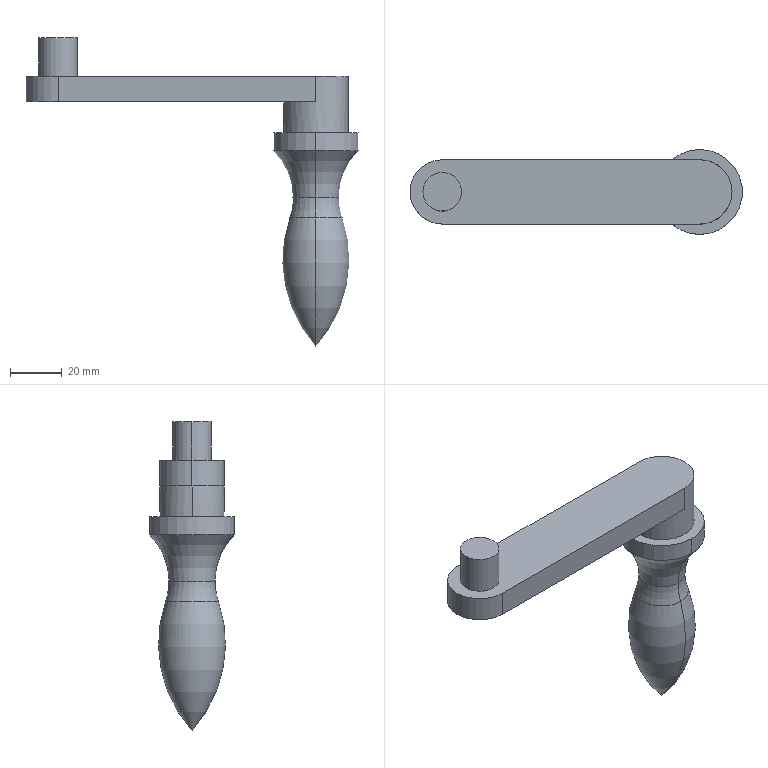Part | SolidWorks | features Extrusion 1, ICE 1, Revolution 1 | 1 solid | 20 faces | box 129 x 33 x 119.886 mm | volume 71552 mm3 | cylinder 8 | torus 6 | plane 6 | commonest cylinder face diameters 25 x4 15 x2 33 x2
STEP:
#1=CARTESIAN_POINT('',(100.,-4.,-19.));
#2=VERTEX_POINT('',#1);
#3=CARTESIAN_POINT('',(100.,3.558,-36.917));
#4=VERTEX_POINT('',#3);
#5=CARTESIAN_POINT('',(100.,-21.456,-36.917));
#6=DIRECTION('',(-1.,0.,0.));
#7=DIRECTION('',(0.,0.,1.));
#8=AXIS2_PLACEMENT_3D('',#5,#6,#7);
#9=CIRCLE('',#8,25.014);
#10=EDGE_CURVE('',#2,#4,#9,.T.);
#11=ORIENTED_EDGE('',*,*,#10,.T.);
#12=CARTESIAN_POINT('',(100.,21.442,-36.917));
#13=VERTEX_POINT('',#12);
#14=CARTESIAN_POINT('',(100.,12.5,-36.917));
#15=DIRECTION('',(0.,0.,1.));
#16=DIRECTION('',(0.,-1.,0.));
#17=AXIS2_PLACEMENT_3D('',#14,#15,#16);
#18=CIRCLE('',#17,8.942);
#19=EDGE_CURVE('',#4,#13,#18,.T.);
#20=ORIENTED_EDGE('',*,*,#19,.T.);
#21=CARTESIAN_POINT('',(100.,29.,-19.));
#22=VERTEX_POINT('',#21);
#23=CARTESIAN_POINT('',(100.,46.456,-36.917));
#24=DIRECTION('',(1.,0.,0.));
#25=DIRECTION('',(0.,1.,0.));
#26=AXIS2_PLACEMENT_3D('',#23,#24,#25);
#27=CIRCLE('',#26,25.014);
#28=EDGE_CURVE('',#22,#13,#27,.T.);
#29=ORIENTED_EDGE('',*,*,#28,.F.);
#30=CARTESIAN_POINT('',(100.,12.5,-19.));
#31=DIRECTION('',(0.,0.,1.));
#32=DIRECTION('',(0.,-1.,0.));
#33=AXIS2_PLACEMENT_3D('',#30,#31,#32);
#34=CIRCLE('',#33,16.5);
#35=EDGE_CURVE('',#2,#22,#34,.T.);
#36=ORIENTED_EDGE('',*,*,#35,.F.);
#37=EDGE_LOOP('',(#11,#20,#29,#36));
#38=FACE_OUTER_BOUND('',#37,.T.);
#39=CARTESIAN_POINT('',(100.,12.5,-36.917));
#40=DIRECTION('',(0.,0.,1.));
#41=DIRECTION('',(0.,-1.,0.));
#42=AXIS2_PLACEMENT_3D('',#39,#40,#41);
#43=TOROIDAL_SURFACE('',#42,33.956,25.014);
#44=ADVANCED_FACE('',(#38),#43,.F.);
#45=ORIENTED_EDGE('',*,*,#28,.T.);
#46=CARTESIAN_POINT('',(100.,12.5,-36.917));
#47=DIRECTION('',(0.,0.,1.));
#48=DIRECTION('',(0.,-1.,0.));
#49=AXIS2_PLACEMENT_3D('',#46,#47,#48);
#50=CIRCLE('',#49,8.942);
#51=EDGE_CURVE('',#13,#4,#50,.T.);
#52=ORIENTED_EDGE('',*,*,#51,.T.);
#53=ORIENTED_EDGE('',*,*,#10,.F.);
#54=CARTESIAN_POINT('',(100.,12.5,-19.));
#55=DIRECTION('',(0.,0.,1.));
#56=DIRECTION('',(0.,-1.,0.));
#57=AXIS2_PLACEMENT_3D('',#54,#55,#56);
#58=CIRCLE('',#57,16.5);
#59=EDGE_CURVE('',#22,#2,#58,.T.);
#60=ORIENTED_EDGE('',*,*,#59,.F.);
#61=EDGE_LOOP('',(#45,#52,#53,#60));
#62=FACE_OUTER_BOUND('',#61,.T.);
#63=CARTESIAN_POINT('',(100.,12.5,-36.917));
#64=DIRECTION('',(0.,0.,1.));
#65=DIRECTION('',(0.,-1.,0.));
#66=AXIS2_PLACEMENT_3D('',#63,#64,#65);
#67=TOROIDAL_SURFACE('',#66,33.956,25.014);
#68=ADVANCED_FACE('',(#62),#67,.F.);
#69=CARTESIAN_POINT('',(100.,12.5,-94.886));
#70=VERTEX_POINT('',#69);
#71=CARTESIAN_POINT('',(100.,2.205,-45.033));
#72=VERTEX_POINT('',#71);
#73=CARTESIAN_POINT('',(100.,49.5,-61.256));
#74=DIRECTION('',(-1.,0.,0.));
#75=DIRECTION('',(0.,0.,1.));
#76=AXIS2_PLACEMENT_3D('',#73,#74,#75);
#77=CIRCLE('',#76,50.);
#78=EDGE_CURVE('',#70,#72,#77,.T.);
#79=ORIENTED_EDGE('',*,*,#78,.F.);
#80=CARTESIAN_POINT('',(100.,22.795,-45.033));
#81=VERTEX_POINT('',#80);
#82=CARTESIAN_POINT('',(100.,-24.5,-61.256));
#83=DIRECTION('',(1.,0.,0.));
#84=DIRECTION('',(0.,1.,0.));
#85=AXIS2_PLACEMENT_3D('',#82,#83,#84);
#86=CIRCLE('',#85,50.);
#87=EDGE_CURVE('',#70,#81,#86,.T.);
#88=ORIENTED_EDGE('',*,*,#87,.T.);
#89=CARTESIAN_POINT('',(100.,12.5,-45.033));
#90=DIRECTION('',(0.,0.,1.));
#91=DIRECTION('',(0.,-1.,0.));
#92=AXIS2_PLACEMENT_3D('',#89,#90,#91);
#93=CIRCLE('',#92,10.295);
#94=EDGE_CURVE('',#72,#81,#93,.T.);
#95=ORIENTED_EDGE('',*,*,#94,.F.);
#96=EDGE_LOOP('',(#79,#88,#95));
#97=FACE_OUTER_BOUND('',#96,.T.);
#98=CARTESIAN_POINT('',(100.,12.5,-61.256));
#99=DIRECTION('',(0.,0.,1.));
#100=DIRECTION('',(0.,-1.,0.));
#101=AXIS2_PLACEMENT_3D('',#98,#99,#100);
#102=TOROIDAL_SURFACE('',#101,-37.,50.);
#103=ADVANCED_FACE('',(#97),#102,.T.);
#104=ORIENTED_EDGE('',*,*,#51,.F.);
#105=CARTESIAN_POINT('',(100.,46.456,-36.917));
#106=DIRECTION('',(1.,0.,0.));
#107=DIRECTION('',(0.,1.,0.));
#108=AXIS2_PLACEMENT_3D('',#105,#106,#107);
#109=CIRCLE('',#108,25.014);
#110=EDGE_CURVE('',#13,#81,#109,.T.);
#111=ORIENTED_EDGE('',*,*,#110,.T.);
#112=CARTESIAN_POINT('',(100.,12.5,-45.033));
#113=DIRECTION('',(0.,0.,1.));
#114=DIRECTION('',(0.,-1.,0.));
#115=AXIS2_PLACEMENT_3D('',#112,#113,#114);
#116=CIRCLE('',#115,10.295);
#117=EDGE_CURVE('',#81,#72,#116,.T.);
#118=ORIENTED_EDGE('',*,*,#117,.T.);
#119=CARTESIAN_POINT('',(100.,-21.456,-36.917));
#120=DIRECTION('',(-1.,0.,0.));
#121=DIRECTION('',(0.,0.,1.));
#122=AXIS2_PLACEMENT_3D('',#119,#120,#121);
#123=CIRCLE('',#122,25.014);
#124=EDGE_CURVE('',#4,#72,#123,.T.);
#125=ORIENTED_EDGE('',*,*,#124,.F.);
#126=EDGE_LOOP('',(#104,#111,#118,#125));
#127=FACE_OUTER_BOUND('',#126,.T.);
#128=CARTESIAN_POINT('',(100.,12.5,-36.917));
#129=DIRECTION('',(0.,0.,1.));
#130=DIRECTION('',(0.,-1.,0.));
#131=AXIS2_PLACEMENT_3D('',#128,#129,#130);
#132=TOROIDAL_SURFACE('',#131,33.956,25.014);
#133=ADVANCED_FACE('',(#127),#132,.F.);
#134=ORIENTED_EDGE('',*,*,#35,.T.);
#135=CARTESIAN_POINT('',(100.,29.,-12.));
#136=VERTEX_POINT('',#135);
#137=CARTESIAN_POINT('',(100.,29.,0.));
#138=DIRECTION('',(0.,0.,1.));
#139=VECTOR('',#138,1000.);
#140=LINE('',#137,#139);
#141=EDGE_CURVE('',#22,#136,#140,.T.);
#142=ORIENTED_EDGE('',*,*,#141,.T.);
#143=CARTESIAN_POINT('',(100.,-4.,-12.));
#144=VERTEX_POINT('',#143);
#145=CARTESIAN_POINT('',(100.,12.5,-12.));
#146=DIRECTION('',(0.,0.,1.));
#147=DIRECTION('',(0.,-1.,0.));
#148=AXIS2_PLACEMENT_3D('',#145,#146,#147);
#149=CIRCLE('',#148,16.5);
#150=EDGE_CURVE('',#144,#136,#149,.T.);
#151=ORIENTED_EDGE('',*,*,#150,.F.);
#152=CARTESIAN_POINT('',(100.,-4.,0.));
#153=DIRECTION('',(0.,0.,1.));
#154=VECTOR('',#153,1000.);
#155=LINE('',#152,#154);
#156=EDGE_CURVE('',#2,#144,#155,.T.);
#157=ORIENTED_EDGE('',*,*,#156,.F.);
#158=EDGE_LOOP('',(#134,#142,#151,#157));
#159=FACE_OUTER_BOUND('',#158,.T.);
#160=CARTESIAN_POINT('',(100.,12.5,0.));
#161=DIRECTION('',(0.,0.,1.));
#162=DIRECTION('',(0.,-1.,0.));
#163=AXIS2_PLACEMENT_3D('',#160,#161,#162);
#164=CYLINDRICAL_SURFACE('',#163,16.5);
#165=ADVANCED_FACE('',(#159),#164,.T.);
#166=CARTESIAN_POINT('',(7.5,12.5,25.));
#167=VERTEX_POINT('',#166);
#168=CARTESIAN_POINT('',(-7.5,12.5,25.));
#169=VERTEX_POINT('',#168);
#170=CARTESIAN_POINT('',(0.,12.5,25.));
#171=DIRECTION('',(0.,0.,1.));
#172=DIRECTION('',(1.,0.,0.));
#173=AXIS2_PLACEMENT_3D('',#170,#171,#172);
#174=CIRCLE('',#173,7.5);
#175=EDGE_CURVE('',#167,#169,#174,.T.);
#176=ORIENTED_EDGE('',*,*,#175,.F.);
#177=CARTESIAN_POINT('',(7.5,12.5,10.));
#178=VERTEX_POINT('',#177);
#179=CARTESIAN_POINT('',(7.5,12.5,25.));
#180=DIRECTION('',(0.,0.,-1.));
#181=VECTOR('',#180,1000.);
#182=LINE('',#179,#181);
#183=EDGE_CURVE('',#167,#178,#182,.T.);
#184=ORIENTED_EDGE('',*,*,#183,.T.);
#185=CARTESIAN_POINT('',(-7.5,12.5,10.));
#186=VERTEX_POINT('',#185);
#187=CARTESIAN_POINT('',(0.,12.5,10.));
#188=DIRECTION('',(0.,0.,1.));
#189=DIRECTION('',(1.,0.,0.));
#190=AXIS2_PLACEMENT_3D('',#187,#188,#189);
#191=CIRCLE('',#190,7.5);
#192=EDGE_CURVE('',#178,#186,#191,.T.);
#193=ORIENTED_EDGE('',*,*,#192,.T.);
#194=CARTESIAN_POINT('',(-7.5,12.5,25.));
#195=DIRECTION('',(0.,0.,-1.));
#196=VECTOR('',#195,1000.);
#197=LINE('',#194,#196);
#198=EDGE_CURVE('',#169,#186,#197,.T.);
#199=ORIENTED_EDGE('',*,*,#198,.F.);
#200=EDGE_LOOP('',(#176,#184,#193,#199));
#201=FACE_OUTER_BOUND('',#200,.T.);
#202=CARTESIAN_POINT('',(0.,12.5,25.));
#203=DIRECTION('',(0.,0.,-1.));
#204=DIRECTION('',(-1.,0.,0.));
#205=AXIS2_PLACEMENT_3D('',#202,#203,#204);
#206=CYLINDRICAL_SURFACE('',#205,7.5);
#207=ADVANCED_FACE('',(#201),#206,.T.);
#208=CARTESIAN_POINT('',(112.5,12.5,10.));
#209=VERTEX_POINT('',#208);
#210=CARTESIAN_POINT('',(100.,25.,10.));
#211=VERTEX_POINT('',#210);
#212=CARTESIAN_POINT('',(100.,12.5,10.));
#213=DIRECTION('',(0.,0.,1.));
#214=DIRECTION('',(1.,0.,0.));
#215=AXIS2_PLACEMENT_3D('',#212,#213,#214);
#216=CIRCLE('',#215,12.5);
#217=EDGE_CURVE('',#209,#211,#216,.T.);
#218=ORIENTED_EDGE('',*,*,#217,.F.);
#219=CARTESIAN_POINT('',(112.5,12.5,-12.));
#220=VERTEX_POINT('',#219);
#221=CARTESIAN_POINT('',(112.5,12.5,10.));
#222=DIRECTION('',(0.,0.,-1.));
#223=VECTOR('',#222,1000.);
#224=LINE('',#221,#223);
#225=EDGE_CURVE('',#209,#220,#224,.T.);
#226=ORIENTED_EDGE('',*,*,#225,.T.);
#227=CARTESIAN_POINT('',(87.5,12.5,-12.));
#228=VERTEX_POINT('',#227);
#229=CARTESIAN_POINT('',(100.,12.5,-12.));
#230=DIRECTION('',(0.,0.,1.));
#231=DIRECTION('',(0.,-1.,0.));
#232=AXIS2_PLACEMENT_3D('',#229,#230,#231);
#233=CIRCLE('',#232,12.5);
#234=EDGE_CURVE('',#220,#228,#233,.T.);
#235=ORIENTED_EDGE('',*,*,#234,.T.);
#236=CARTESIAN_POINT('',(87.5,12.5,0.));
#237=VERTEX_POINT('',#236);
#238=CARTESIAN_POINT('',(87.5,12.5,10.));
#239=DIRECTION('',(0.,0.,-1.));
#240=VECTOR('',#239,1000.);
#241=LINE('',#238,#240);
#242=EDGE_CURVE('',#237,#228,#241,.T.);
#243=ORIENTED_EDGE('',*,*,#242,.F.);
#244=CARTESIAN_POINT('',(100.,25.,0.));
#245=VERTEX_POINT('',#244);
#246=CARTESIAN_POINT('',(100.,12.5,0.));
#247=DIRECTION('',(0.,0.,1.));
#248=DIRECTION('',(0.,-1.,0.));
#249=AXIS2_PLACEMENT_3D('',#246,#247,#248);
#250=CIRCLE('',#249,12.5);
#251=EDGE_CURVE('',#245,#237,#250,.T.);
#252=ORIENTED_EDGE('',*,*,#251,.F.);
#253=CARTESIAN_POINT('',(100.,25.,10.));
#254=DIRECTION('',(0.,0.,-1.));
#255=VECTOR('',#254,1000.);
#256=LINE('',#253,#255);
#257=EDGE_CURVE('',#211,#245,#256,.T.);
#258=ORIENTED_EDGE('',*,*,#257,.F.);
#259=EDGE_LOOP('',(#218,#226,#235,#243,#252,#258));
#260=FACE_OUTER_BOUND('',#259,.T.);
#261=CARTESIAN_POINT('',(100.,12.5,10.));
#262=DIRECTION('',(0.,0.,-1.));
#263=DIRECTION('',(-1.,0.,0.));
#264=AXIS2_PLACEMENT_3D('',#261,#262,#263);
#265=CYLINDRICAL_SURFACE('',#264,12.5);
#266=ADVANCED_FACE('',(#260),#265,.T.);
#267=CARTESIAN_POINT('',(-12.5,12.5,10.));
#268=VERTEX_POINT('',#267);
#269=CARTESIAN_POINT('',(0.,0.,10.));
#270=VERTEX_POINT('',#269);
#271=CARTESIAN_POINT('',(0.,12.5,10.));
#272=DIRECTION('',(0.,0.,1.));
#273=DIRECTION('',(1.,0.,0.));
#274=AXIS2_PLACEMENT_3D('',#271,#272,#273);
#275=CIRCLE('',#274,12.5);
#276=EDGE_CURVE('',#268,#270,#275,.T.);
#277=ORIENTED_EDGE('',*,*,#276,.F.);
#278=CARTESIAN_POINT('',(-12.5,12.5,0.));
#279=VERTEX_POINT('',#278);
#280=CARTESIAN_POINT('',(-12.5,12.5,10.));
#281=DIRECTION('',(0.,0.,-1.));
#282=VECTOR('',#281,1000.);
#283=LINE('',#280,#282);
#284=EDGE_CURVE('',#268,#279,#283,.T.);
#285=ORIENTED_EDGE('',*,*,#284,.T.);
#286=CARTESIAN_POINT('',(0.,0.,0.));
#287=VERTEX_POINT('',#286);
#288=CARTESIAN_POINT('',(0.,12.5,0.));
#289=DIRECTION('',(0.,0.,1.));
#290=DIRECTION('',(1.,0.,0.));
#291=AXIS2_PLACEMENT_3D('',#288,#289,#290);
#292=CIRCLE('',#291,12.5);
#293=EDGE_CURVE('',#279,#287,#292,.T.);
#294=ORIENTED_EDGE('',*,*,#293,.T.);
#295=CARTESIAN_POINT('',(0.,0.,10.));
#296=DIRECTION('',(0.,0.,-1.));
#297=VECTOR('',#296,1000.);
#298=LINE('',#295,#297);
#299=EDGE_CURVE('',#270,#287,#298,.T.);
#300=ORIENTED_EDGE('',*,*,#299,.F.);
#301=EDGE_LOOP('',(#277,#285,#294,#300));
#302=FACE_OUTER_BOUND('',#301,.T.);
#303=CARTESIAN_POINT('',(0.,12.5,10.));
#304=DIRECTION('',(0.,0.,-1.));
#305=DIRECTION('',(-1.,0.,0.));
#306=AXIS2_PLACEMENT_3D('',#303,#304,#305);
#307=CYLINDRICAL_SURFACE('',#306,12.5);
#308=ADVANCED_FACE('',(#302),#307,.T.);
#309=CARTESIAN_POINT('',(0.,25.,10.));
#310=VERTEX_POINT('',#309);
#311=CARTESIAN_POINT('',(0.,12.5,10.));
#312=DIRECTION('',(0.,0.,1.));
#313=DIRECTION('',(1.,0.,0.));
#314=AXIS2_PLACEMENT_3D('',#311,#312,#313);
#315=CIRCLE('',#314,12.5);
#316=EDGE_CURVE('',#310,#268,#315,.T.);
#317=ORIENTED_EDGE('',*,*,#316,.T.);
#318=ORIENTED_EDGE('',*,*,#276,.T.);
#319=CARTESIAN_POINT('',(100.,0.,10.));
#320=VERTEX_POINT('',#319);
#321=CARTESIAN_POINT('',(0.,0.,10.));
#322=DIRECTION('',(1.,0.,0.));
#323=VECTOR('',#322,1000.);
#324=LINE('',#321,#323);
#325=EDGE_CURVE('',#270,#320,#324,.T.);
#326=ORIENTED_EDGE('',*,*,#325,.T.);
#327=CARTESIAN_POINT('',(100.,12.5,10.));
#328=DIRECTION('',(0.,0.,1.));
#329=DIRECTION('',(1.,0.,0.));
#330=AXIS2_PLACEMENT_3D('',#327,#328,#329);
#331=CIRCLE('',#330,12.5);
#332=EDGE_CURVE('',#320,#209,#331,.T.);
#333=ORIENTED_EDGE('',*,*,#332,.T.);
#334=ORIENTED_EDGE('',*,*,#217,.T.);
#335=CARTESIAN_POINT('',(0.,25.,10.));
#336=DIRECTION('',(-1.,0.,0.));
#337=VECTOR('',#336,1000.);
#338=LINE('',#335,#337);
#339=EDGE_CURVE('',#211,#310,#338,.T.);
#340=ORIENTED_EDGE('',*,*,#339,.T.);
#341=EDGE_LOOP('',(#317,#318,#326,#333,#334,#340));
#342=FACE_OUTER_BOUND('',#341,.T.);
#343=CARTESIAN_POINT('',(0.,12.5,10.));
#344=DIRECTION('',(0.,0.,1.));
#345=DIRECTION('',(1.,0.,0.));
#346=AXIS2_PLACEMENT_3D('',#343,#344,#345);
#347=CIRCLE('',#346,7.5);
#348=EDGE_CURVE('',#186,#178,#347,.T.);
#349=ORIENTED_EDGE('',*,*,#348,.F.);
#350=ORIENTED_EDGE('',*,*,#192,.F.);
#351=EDGE_LOOP('',(#349,#350));
#352=FACE_BOUND('',#351,.T.);
#353=CARTESIAN_POINT('',(0.,12.5,10.));
#354=DIRECTION('',(0.,0.,1.));
#355=DIRECTION('',(1.,0.,0.));
#356=AXIS2_PLACEMENT_3D('',#353,#354,#355);
#357=PLANE('',#356);
#358=ADVANCED_FACE('',(#342,#352),#357,.T.);
#359=ORIENTED_EDGE('',*,*,#284,.F.);
#360=ORIENTED_EDGE('',*,*,#316,.F.);
#361=CARTESIAN_POINT('',(0.,25.,0.));
#362=VERTEX_POINT('',#361);
#363=CARTESIAN_POINT('',(0.,25.,10.));
#364=DIRECTION('',(0.,0.,-1.));
#365=VECTOR('',#364,1000.);
#366=LINE('',#363,#365);
#367=EDGE_CURVE('',#310,#362,#366,.T.);
#368=ORIENTED_EDGE('',*,*,#367,.T.);
#369=CARTESIAN_POINT('',(0.,12.5,0.));
#370=DIRECTION('',(0.,0.,1.));
#371=DIRECTION('',(1.,0.,0.));
#372=AXIS2_PLACEMENT_3D('',#369,#370,#371);
#373=CIRCLE('',#372,12.5);
#374=EDGE_CURVE('',#362,#279,#373,.T.);
#375=ORIENTED_EDGE('',*,*,#374,.T.);
#376=EDGE_LOOP('',(#359,#360,#368,#375));
#377=FACE_OUTER_BOUND('',#376,.T.);
#378=CARTESIAN_POINT('',(0.,12.5,10.));
#379=DIRECTION('',(0.,0.,-1.));
#380=DIRECTION('',(-1.,0.,0.));
#381=AXIS2_PLACEMENT_3D('',#378,#379,#380);
#382=CYLINDRICAL_SURFACE('',#381,12.5);
#383=ADVANCED_FACE('',(#377),#382,.T.);
#384=CARTESIAN_POINT('',(100.,0.,0.));
#385=VERTEX_POINT('',#384);
#386=CARTESIAN_POINT('',(0.,0.,0.));
#387=DIRECTION('',(1.,0.,0.));
#388=VECTOR('',#387,1000.);
#389=LINE('',#386,#388);
#390=EDGE_CURVE('',#287,#385,#389,.T.);
#391=ORIENTED_EDGE('',*,*,#390,.T.);
#392=CARTESIAN_POINT('',(100.,0.,10.));
#393=DIRECTION('',(0.,0.,-1.));
#394=VECTOR('',#393,1000.);
#395=LINE('',#392,#394);
#396=EDGE_CURVE('',#320,#385,#395,.T.);
#397=ORIENTED_EDGE('',*,*,#396,.F.);
#398=ORIENTED_EDGE('',*,*,#325,.F.);
#399=ORIENTED_EDGE('',*,*,#299,.T.);
#400=EDGE_LOOP('',(#391,#397,#398,#399));
#401=FACE_OUTER_BOUND('',#400,.T.);
#402=CARTESIAN_POINT('',(0.,0.,10.));
#403=DIRECTION('',(0.,1.,0.));
#404=DIRECTION('',(0.,0.,1.));
#405=AXIS2_PLACEMENT_3D('',#402,#403,#404);
#406=PLANE('',#405);
#407=ADVANCED_FACE('',(#401),#406,.F.);
#408=ORIENTED_EDGE('',*,*,#225,.F.);
#409=ORIENTED_EDGE('',*,*,#332,.F.);
#410=ORIENTED_EDGE('',*,*,#396,.T.);
#411=CARTESIAN_POINT('',(100.,12.5,0.));
#412=DIRECTION('',(0.,0.,1.));
#413=DIRECTION('',(0.,-1.,0.));
#414=AXIS2_PLACEMENT_3D('',#411,#412,#413);
#415=CIRCLE('',#414,12.5);
#416=EDGE_CURVE('',#237,#385,#415,.T.);
#417=ORIENTED_EDGE('',*,*,#416,.F.);
#418=ORIENTED_EDGE('',*,*,#242,.T.);
#419=CARTESIAN_POINT('',(100.,12.5,-12.));
#420=DIRECTION('',(0.,0.,1.));
#421=DIRECTION('',(0.,-1.,0.));
#422=AXIS2_PLACEMENT_3D('',#419,#420,#421);
#423=CIRCLE('',#422,12.5);
#424=EDGE_CURVE('',#228,#220,#423,.T.);
#425=ORIENTED_EDGE('',*,*,#424,.T.);
#426=EDGE_LOOP('',(#408,#409,#410,#417,#418,#425));
#427=FACE_OUTER_BOUND('',#426,.T.);
#428=CARTESIAN_POINT('',(100.,12.5,10.));
#429=DIRECTION('',(0.,0.,-1.));
#430=DIRECTION('',(-1.,0.,0.));
#431=AXIS2_PLACEMENT_3D('',#428,#429,#430);
#432=CYLINDRICAL_SURFACE('',#431,12.5);
#433=ADVANCED_FACE('',(#427),#432,.T.);
#434=CARTESIAN_POINT('',(0.,25.,0.));
#435=DIRECTION('',(-1.,0.,0.));
#436=VECTOR('',#435,1000.);
#437=LINE('',#434,#436);
#438=EDGE_CURVE('',#245,#362,#437,.T.);
#439=ORIENTED_EDGE('',*,*,#438,.T.);
#440=ORIENTED_EDGE('',*,*,#367,.F.);
#441=ORIENTED_EDGE('',*,*,#339,.F.);
#442=ORIENTED_EDGE('',*,*,#257,.T.);
#443=EDGE_LOOP('',(#439,#440,#441,#442));
#444=FACE_OUTER_BOUND('',#443,.T.);
#445=CARTESIAN_POINT('',(0.,25.,10.));
#446=DIRECTION('',(0.,-1.,0.));
#447=DIRECTION('',(0.,0.,-1.));
#448=AXIS2_PLACEMENT_3D('',#445,#446,#447);
#449=PLANE('',#448);
#450=ADVANCED_FACE('',(#444),#449,.F.);
#451=ORIENTED_EDGE('',*,*,#438,.F.);
#452=ORIENTED_EDGE('',*,*,#251,.T.);
#453=ORIENTED_EDGE('',*,*,#416,.T.);
#454=ORIENTED_EDGE('',*,*,#390,.F.);
#455=ORIENTED_EDGE('',*,*,#293,.F.);
#456=ORIENTED_EDGE('',*,*,#374,.F.);
#457=EDGE_LOOP('',(#451,#452,#453,#454,#455,#456));
#458=FACE_OUTER_BOUND('',#457,.T.);
#459=CARTESIAN_POINT('',(0.,12.5,0.));
#460=DIRECTION('',(0.,0.,1.));
#461=DIRECTION('',(1.,0.,0.));
#462=AXIS2_PLACEMENT_3D('',#459,#460,#461);
#463=PLANE('',#462);
#464=ADVANCED_FACE('',(#458),#463,.F.);
#465=ORIENTED_EDGE('',*,*,#183,.F.);
#466=CARTESIAN_POINT('',(0.,12.5,25.));
#467=DIRECTION('',(0.,0.,1.));
#468=DIRECTION('',(1.,0.,0.));
#469=AXIS2_PLACEMENT_3D('',#466,#467,#468);
#470=CIRCLE('',#469,7.5);
#471=EDGE_CURVE('',#169,#167,#470,.T.);
#472=ORIENTED_EDGE('',*,*,#471,.F.);
#473=ORIENTED_EDGE('',*,*,#198,.T.);
#474=ORIENTED_EDGE('',*,*,#348,.T.);
#475=EDGE_LOOP('',(#465,#472,#473,#474));
#476=FACE_OUTER_BOUND('',#475,.T.);
#477=CARTESIAN_POINT('',(0.,12.5,25.));
#478=DIRECTION('',(0.,0.,-1.));
#479=DIRECTION('',(-1.,0.,0.));
#480=AXIS2_PLACEMENT_3D('',#477,#478,#479);
#481=CYLINDRICAL_SURFACE('',#480,7.5);
#482=ADVANCED_FACE('',(#476),#481,.T.);
#483=ORIENTED_EDGE('',*,*,#471,.T.);
#484=ORIENTED_EDGE('',*,*,#175,.T.);
#485=EDGE_LOOP('',(#483,#484));
#486=FACE_OUTER_BOUND('',#485,.T.);
#487=CARTESIAN_POINT('',(0.,12.5,25.));
#488=DIRECTION('',(0.,0.,1.));
#489=DIRECTION('',(1.,0.,0.));
#490=AXIS2_PLACEMENT_3D('',#487,#488,#489);
#491=PLANE('',#490);
#492=ADVANCED_FACE('',(#486),#491,.T.);
#493=ORIENTED_EDGE('',*,*,#424,.F.);
#494=ORIENTED_EDGE('',*,*,#234,.F.);
#495=EDGE_LOOP('',(#493,#494));
#496=FACE_BOUND('',#495,.T.);
#497=ORIENTED_EDGE('',*,*,#150,.T.);
#498=CARTESIAN_POINT('',(100.,12.5,-12.));
#499=DIRECTION('',(0.,0.,1.));
#500=DIRECTION('',(0.,-1.,0.));
#501=AXIS2_PLACEMENT_3D('',#498,#499,#500);
#502=CIRCLE('',#501,16.5);
#503=EDGE_CURVE('',#136,#144,#502,.T.);
#504=ORIENTED_EDGE('',*,*,#503,.T.);
#505=EDGE_LOOP('',(#497,#504));
#506=FACE_OUTER_BOUND('',#505,.T.);
#507=CARTESIAN_POINT('',(100.,25.,-12.));
#508=DIRECTION('',(0.,0.,-1.));
#509=DIRECTION('',(0.,1.,0.));
#510=AXIS2_PLACEMENT_3D('',#507,#508,#509);
#511=PLANE('',#510);
#512=ADVANCED_FACE('',(#496,#506),#511,.F.);
#513=ORIENTED_EDGE('',*,*,#141,.F.);
#514=ORIENTED_EDGE('',*,*,#59,.T.);
#515=ORIENTED_EDGE('',*,*,#156,.T.);
#516=ORIENTED_EDGE('',*,*,#503,.F.);
#517=EDGE_LOOP('',(#513,#514,#515,#516));
#518=FACE_OUTER_BOUND('',#517,.T.);
#519=CARTESIAN_POINT('',(100.,12.5,0.));
#520=DIRECTION('',(0.,0.,1.));
#521=DIRECTION('',(0.,-1.,0.));
#522=AXIS2_PLACEMENT_3D('',#519,#520,#521);
#523=CYLINDRICAL_SURFACE('',#522,16.5);
#524=ADVANCED_FACE('',(#518),#523,.T.);
#525=ORIENTED_EDGE('',*,*,#19,.F.);
#526=ORIENTED_EDGE('',*,*,#124,.T.);
#527=ORIENTED_EDGE('',*,*,#94,.T.);
#528=ORIENTED_EDGE('',*,*,#110,.F.);
#529=EDGE_LOOP('',(#525,#526,#527,#528));
#530=FACE_OUTER_BOUND('',#529,.T.);
#531=CARTESIAN_POINT('',(100.,12.5,-36.917));
#532=DIRECTION('',(0.,0.,1.));
#533=DIRECTION('',(0.,-1.,0.));
#534=AXIS2_PLACEMENT_3D('',#531,#532,#533);
#535=TOROIDAL_SURFACE('',#534,33.956,25.014);
#536=ADVANCED_FACE('',(#530),#535,.F.);
#537=ORIENTED_EDGE('',*,*,#87,.F.);
#538=ORIENTED_EDGE('',*,*,#78,.T.);
#539=ORIENTED_EDGE('',*,*,#117,.F.);
#540=EDGE_LOOP('',(#537,#538,#539));
#541=FACE_OUTER_BOUND('',#540,.T.);
#542=CARTESIAN_POINT('',(100.,12.5,-61.256));
#543=DIRECTION('',(0.,0.,1.));
#544=DIRECTION('',(0.,-1.,0.));
#545=AXIS2_PLACEMENT_3D('',#542,#543,#544);
#546=TOROIDAL_SURFACE('',#545,-37.,50.);
#547=ADVANCED_FACE('',(#541),#546,.T.);
#548=CLOSED_SHELL('',(#44,#68,#103,#133,#165,#207,#266,#308,#358,#383,#407,#433,#450,#464,#482,#492,#512,#524,#536,#547));
#549=MANIFOLD_SOLID_BREP('',#548);
#550=CARTESIAN_POINT('',(0.,0.,0.));
#551=DIRECTION('',(0.,0.,1.));
#552=DIRECTION('',(1.,0.,0.));
#553=AXIS2_PLACEMENT_3D('',#550,#551,#552);
#554=(LENGTH_UNIT()NAMED_UNIT(*)SI_UNIT(.MILLI.,.METRE.));
#555=UNCERTAINTY_MEASURE_WITH_UNIT(LENGTH_MEASURE(0.00001),#554,'','');
#556=(NAMED_UNIT(*)PLANE_ANGLE_UNIT()SI_UNIT($,.RADIAN.));
#557=(NAMED_UNIT(*)SI_UNIT($,.STERADIAN.)SOLID_ANGLE_UNIT());
#558=(GEOMETRIC_REPRESENTATION_CONTEXT(3)GLOBAL_UNCERTAINTY_ASSIGNED_CONTEXT((#555))GLOBAL_UNIT_ASSIGNED_CONTEXT((#554,#556,#557))REPRESENTATION_CONTEXT('',''));
#559=ADVANCED_BREP_SHAPE_REPRESENTATION('',(#549,#553),#558);